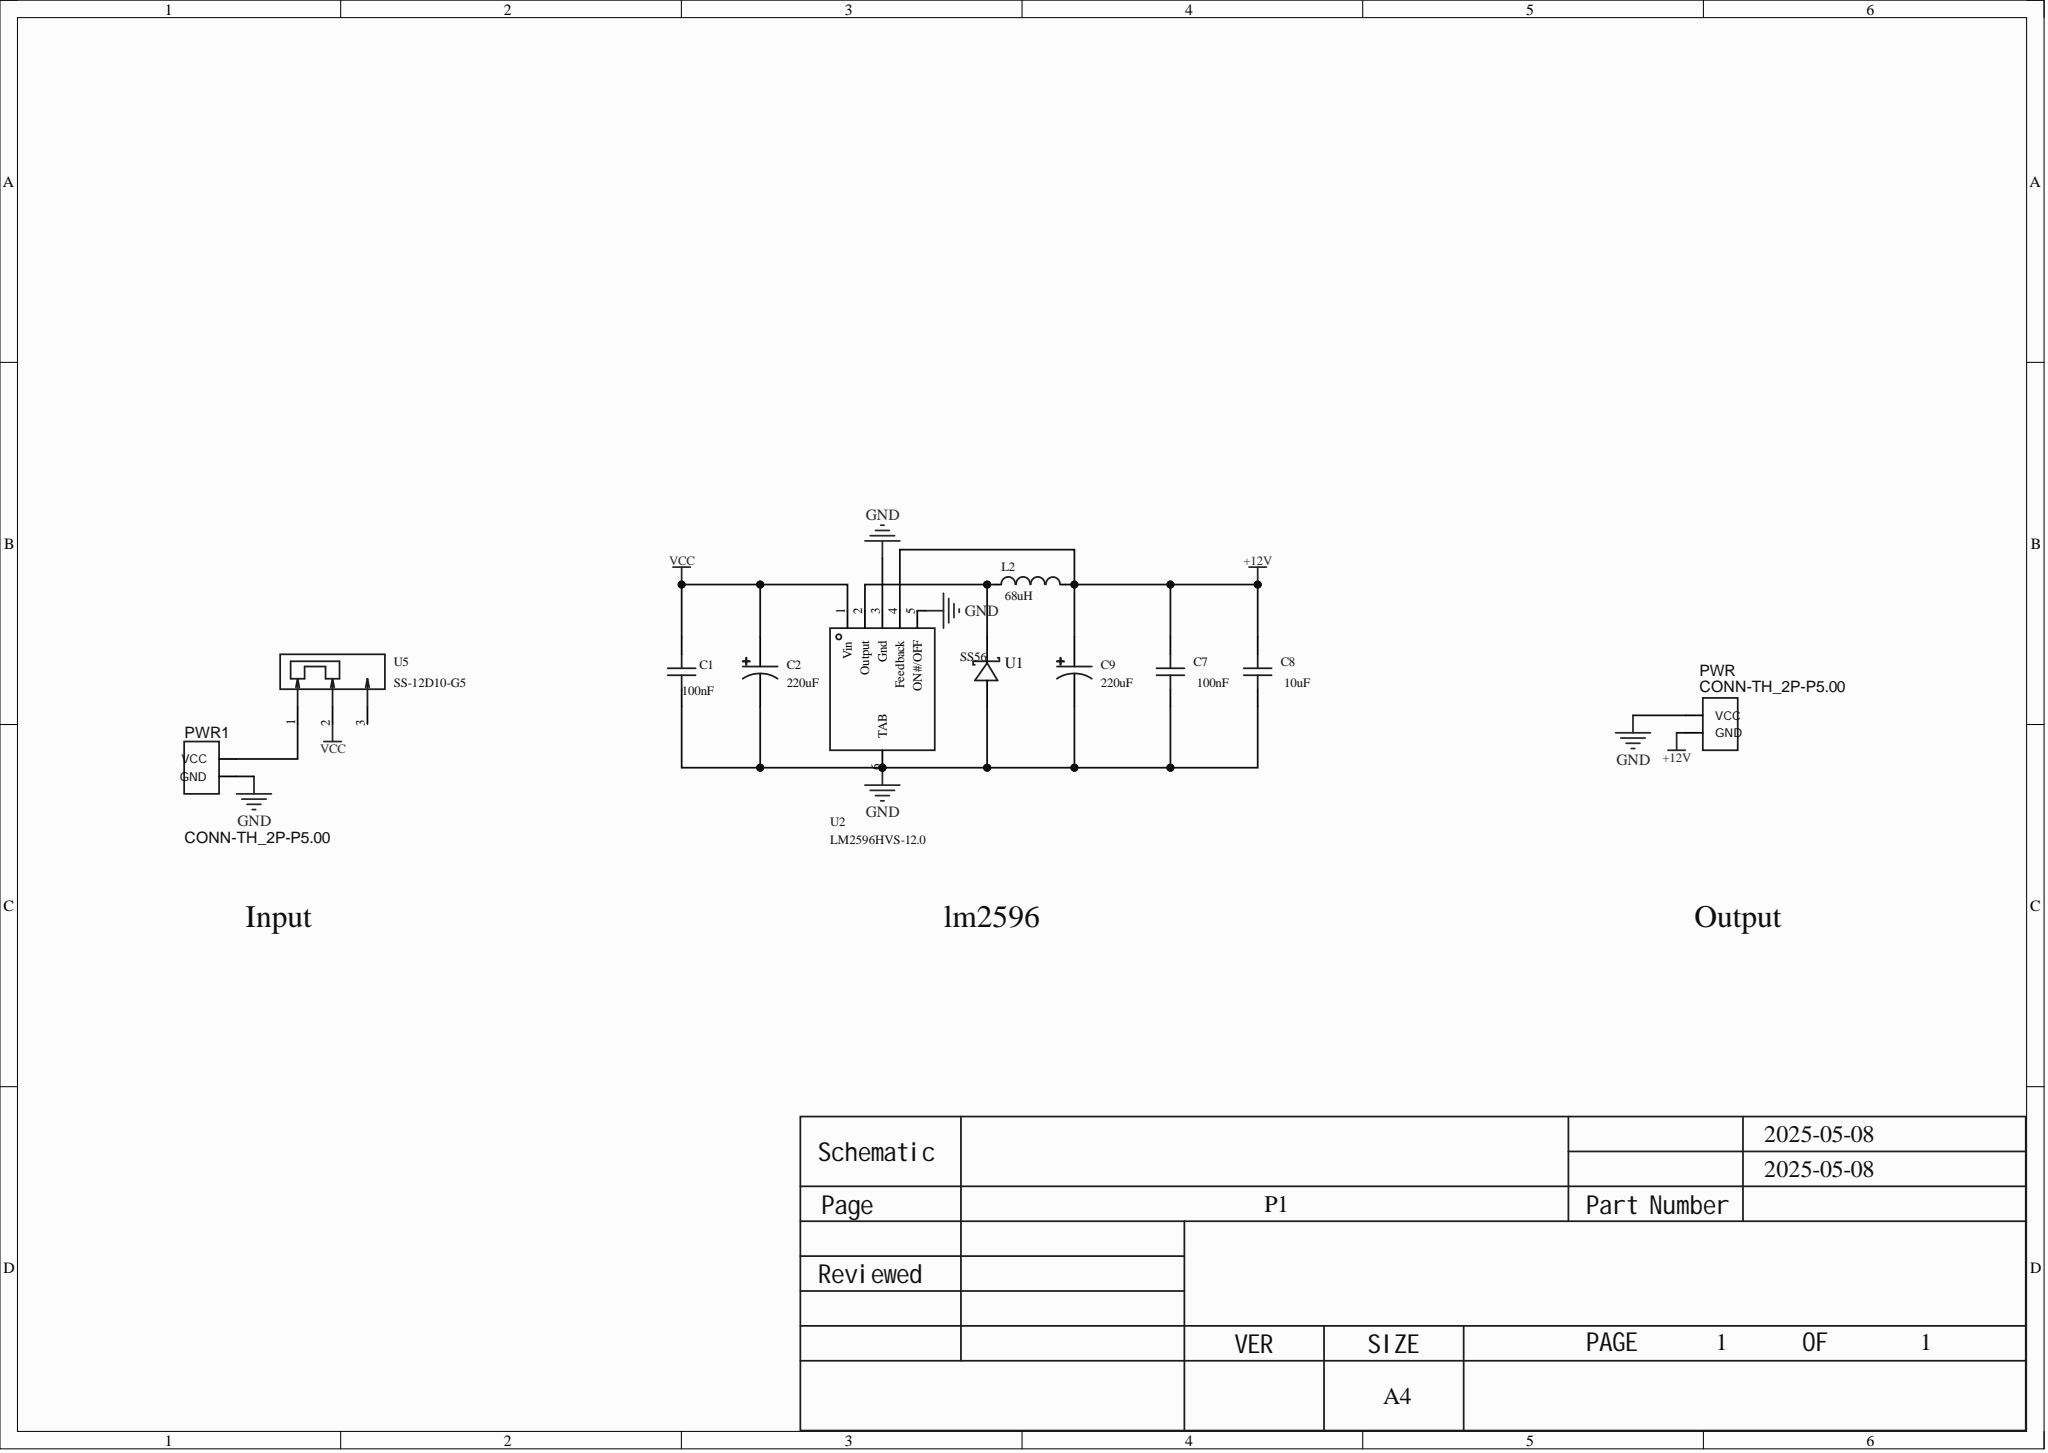Circuit board | Altium Designer | 11 parts | 5 nets
Bill of materials:
Comment,Description,Designator,Footprint,LibRef,Quantity
"100nF","","C1, C7","C1206","CAP_0603, CAP_1206","2"
"220uF","Capacitance:2200uF;Tolerance:±20%;Rated voltage:10V;Body diameter:12.5mm;Body length:13.5mm;Ripple current:-;ESR:-;Life:2000hrs@105℃;Operating temperature:-45℃~+105℃;","C2","CAP-SMD_BD10.0-L10.3-W10.3-FD-LS11.3","VEJ222M1ATR-1313","1"
"10uF","","C8","C0805","CAP_0805","1"
"220uF","Capacitance:2200uF;Tolerance:±20%;Rated voltage:10V;Body diameter:12.5mm;Body length:13.5mm;Ripple current:-;ESR:-;Life:2000hrs@105℃;Operating temperature:-45℃~+105℃;","C9","CAP-SMD_BD8.0-L8.3-W8.3-FD-1","VEJ222M1ATR-1313","1"
"68uH","","L2","IND-SMD_L12.0-W12.0_744771008","L_0603","1"
"CONN-TH_2P-P5.00","","PWR, PWR1","CONN-TH_2P-P5.00","CONN-TH_2P-P5.00","2"
"SS56","DC reverse voltage (Vr):60V;Average rectified current (Io):5A;Forward voltage (Vf):700mV@5A;Reverse current (Ir):1mA@60V;","U1","SMC_L6.9-W5.9-LS7.9-RD","SS56_C2931905","1"
"LM2596HVS-12.0","","U2","TO-263-5_L10.0-W8.4-P1.70-LS15.3-BR","LM2596HVS-5.0","1"
"SS-12D10-G5","","U5","SW-TH_SS-12D10-G050","SS-12D10-G5","1"
Netlist (Protel format):
[
C1
C1206
100nF



]
[
C2
CAP-SMD_BD10.0-L10.3-W10.3-FD-LS11.3
220uF



]
[
C7
C1206
100nF



]
[
C8
C0805
10uF



]
[
C9
CAP-SMD_BD8.0-L8.3-W8.3-FD-1
220uF



]
[
L2
IND-SMD_L12.0-W12.0_744771008
68uH



]
[
PWR
CONN-TH_2P-P5.00
CONN-TH_2P-P5.00



]
[
PWR1
CONN-TH_2P-P5.00
CONN-TH_2P-P5.00



]
[
U1
SMC_L6.9-W5.9-LS7.9-RD
SS56



]
[
U2
TO-263-5_L10.0-W8.4-P1.70-LS15.3-BR
LM2596HVS-12.0



]
[
U5
SW-TH_SS-12D10-G050
SS-12D10-G5



]
(
VCC
C1-2
C2-1
U2-1
U5-2
)
(
NetPWR1_1
PWR1-1
U5-1
)
(
NetL2_1
L2-1
U1-1
U2-2
)
(
GND
C1-1
C2-2
C7-1
C8-1
C9-2
PWR-1
PWR1-2
U1-2
U2-3
U2-5
U2-6
)
(
+12V
C7-2
C8-2
C9-1
L2-2
PWR-2
U2-4
)